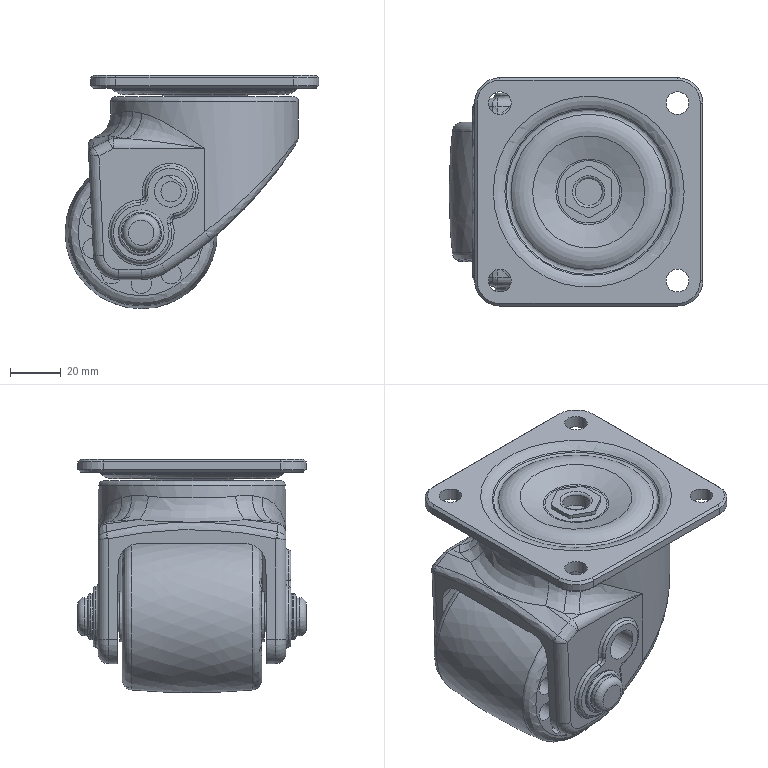Part | STEP file | GLH-60-ASF | 1 solid | 353 faces | box 100 x 90 x 92 mm | volume 321084 mm3 | plane 109 | spline 93 | cylinder 65 | cone 37 | torus 29 | sphere 20 | commonest cylinder face diameters 8 x26 20 x9 4 x6 9 x4 11.95 x2 12.2 x2